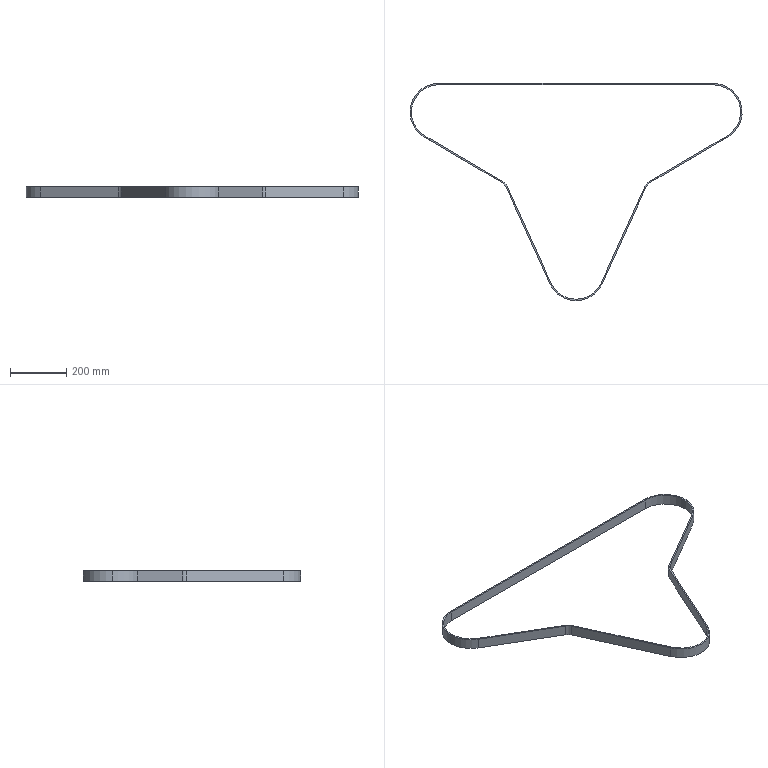Part | SolidWorks | features BeltProfileFeature 1, ExtruThin 1 | 1 solid | 24 faces | box 1186 x 775.76 x 38 mm | volume 604622 mm3 | cylinder 12 | plane 12 | commonest cylinder face diameters 195.76 x4 205.76 x4 65 x2 75 x2
STEP:
#1=CARTESIAN_POINT('',(-490.,667.88,19.));
#2=VERTEX_POINT('',#1);
#3=CARTESIAN_POINT('',(-587.88,570.,19.));
#4=VERTEX_POINT('',#3);
#5=CARTESIAN_POINT('',(-490.,570.,19.));
#6=DIRECTION('',(0.,0.,1.));
#7=DIRECTION('',(-1.,0.,0.));
#8=AXIS2_PLACEMENT_3D('',#5,#6,#7);
#9=CIRCLE('',#8,97.88);
#10=EDGE_CURVE('',#2,#4,#9,.T.);
#11=ORIENTED_EDGE('',*,*,#10,.T.);
#12=CARTESIAN_POINT('',(-587.88,570.,-19.));
#13=VERTEX_POINT('',#12);
#14=CARTESIAN_POINT('',(-587.88,570.,19.));
#15=DIRECTION('',(0.,0.,-1.));
#16=VECTOR('',#15,1000.);
#17=LINE('',#14,#16);
#18=EDGE_CURVE('',#4,#13,#17,.T.);
#19=ORIENTED_EDGE('',*,*,#18,.T.);
#20=CARTESIAN_POINT('',(-490.,667.88,-19.));
#21=VERTEX_POINT('',#20);
#22=CARTESIAN_POINT('',(-490.,570.,-19.));
#23=DIRECTION('',(0.,0.,1.));
#24=DIRECTION('',(-1.,0.,0.));
#25=AXIS2_PLACEMENT_3D('',#22,#23,#24);
#26=CIRCLE('',#25,97.88);
#27=EDGE_CURVE('',#21,#13,#26,.T.);
#28=ORIENTED_EDGE('',*,*,#27,.F.);
#29=CARTESIAN_POINT('',(-490.,667.88,19.));
#30=DIRECTION('',(0.,0.,-1.));
#31=VECTOR('',#30,1000.);
#32=LINE('',#29,#31);
#33=EDGE_CURVE('',#2,#21,#32,.T.);
#34=ORIENTED_EDGE('',*,*,#33,.F.);
#35=EDGE_LOOP('',(#11,#19,#28,#34));
#36=FACE_OUTER_BOUND('',#35,.T.);
#37=CARTESIAN_POINT('',(-490.,570.,19.));
#38=DIRECTION('',(0.,0.,-1.));
#39=DIRECTION('',(-1.,0.,0.));
#40=AXIS2_PLACEMENT_3D('',#37,#38,#39);
#41=CYLINDRICAL_SURFACE('',#40,97.88);
#42=ADVANCED_FACE('',(#36),#41,.F.);
#43=CARTESIAN_POINT('',(-592.88,570.,19.));
#44=VERTEX_POINT('',#43);
#45=CARTESIAN_POINT('',(-542.021,481.241,19.));
#46=VERTEX_POINT('',#45);
#47=CARTESIAN_POINT('',(-490.,570.,19.));
#48=DIRECTION('',(0.,0.,1.));
#49=DIRECTION('',(-1.,0.,0.));
#50=AXIS2_PLACEMENT_3D('',#47,#48,#49);
#51=CIRCLE('',#50,102.88);
#52=EDGE_CURVE('',#44,#46,#51,.T.);
#53=ORIENTED_EDGE('',*,*,#52,.F.);
#54=CARTESIAN_POINT('',(-592.88,570.,-19.));
#55=VERTEX_POINT('',#54);
#56=CARTESIAN_POINT('',(-592.88,570.,19.));
#57=DIRECTION('',(0.,0.,-1.));
#58=VECTOR('',#57,1000.);
#59=LINE('',#56,#58);
#60=EDGE_CURVE('',#44,#55,#59,.T.);
#61=ORIENTED_EDGE('',*,*,#60,.T.);
#62=CARTESIAN_POINT('',(-542.021,481.241,-19.));
#63=VERTEX_POINT('',#62);
#64=CARTESIAN_POINT('',(-490.,570.,-19.));
#65=DIRECTION('',(0.,0.,1.));
#66=DIRECTION('',(-1.,0.,0.));
#67=AXIS2_PLACEMENT_3D('',#64,#65,#66);
#68=CIRCLE('',#67,102.88);
#69=EDGE_CURVE('',#55,#63,#68,.T.);
#70=ORIENTED_EDGE('',*,*,#69,.T.);
#71=CARTESIAN_POINT('',(-542.021,481.241,19.));
#72=DIRECTION('',(0.,0.,-1.));
#73=VECTOR('',#72,1000.);
#74=LINE('',#71,#73);
#75=EDGE_CURVE('',#46,#63,#74,.T.);
#76=ORIENTED_EDGE('',*,*,#75,.F.);
#77=EDGE_LOOP('',(#53,#61,#70,#76));
#78=FACE_OUTER_BOUND('',#77,.T.);
#79=CARTESIAN_POINT('',(-490.,570.,19.));
#80=DIRECTION('',(0.,0.,-1.));
#81=DIRECTION('',(-1.,0.,0.));
#82=AXIS2_PLACEMENT_3D('',#79,#80,#81);
#83=CYLINDRICAL_SURFACE('',#82,102.88);
#84=ADVANCED_FACE('',(#78),#83,.T.);
#85=CARTESIAN_POINT('',(-93.712,-42.454,19.));
#86=VERTEX_POINT('',#85);
#87=CARTESIAN_POINT('',(93.712,-42.454,19.));
#88=VERTEX_POINT('',#87);
#89=CARTESIAN_POINT('',(0.,-0.00002578,19.));
#90=DIRECTION('',(0.,0.,1.));
#91=DIRECTION('',(-1.,0.,0.));
#92=AXIS2_PLACEMENT_3D('',#89,#90,#91);
#93=CIRCLE('',#92,102.88);
#94=EDGE_CURVE('',#86,#88,#93,.T.);
#95=ORIENTED_EDGE('',*,*,#94,.T.);
#96=CARTESIAN_POINT('',(250.396,303.411,19.));
#97=VERTEX_POINT('',#96);
#98=CARTESIAN_POINT('',(93.712,-42.454,19.));
#99=DIRECTION('',(0.4127,0.9109,0.));
#100=VECTOR('',#99,1000.);
#101=LINE('',#98,#100);
#102=EDGE_CURVE('',#88,#97,#101,.T.);
#103=ORIENTED_EDGE('',*,*,#102,.T.);
#104=CARTESIAN_POINT('',(263.566,318.039,19.));
#105=VERTEX_POINT('',#104);
#106=CARTESIAN_POINT('',(280.,290.,19.));
#107=DIRECTION('',(0.,0.,-1.));
#108=DIRECTION('',(-1.,0.,0.));
#109=AXIS2_PLACEMENT_3D('',#106,#107,#108);
#110=CIRCLE('',#109,32.5);
#111=EDGE_CURVE('',#97,#105,#110,.T.);
#112=ORIENTED_EDGE('',*,*,#111,.T.);
#113=CARTESIAN_POINT('',(542.021,481.241,19.));
#114=VERTEX_POINT('',#113);
#115=CARTESIAN_POINT('',(-71.353,121.743,19.));
#116=DIRECTION('',(0.8627,0.5057,0.));
#117=VECTOR('',#116,1000.);
#118=LINE('',#115,#117);
#119=EDGE_CURVE('',#105,#114,#118,.T.);
#120=ORIENTED_EDGE('',*,*,#119,.T.);
#121=CARTESIAN_POINT('',(490.,672.88,19.));
#122=VERTEX_POINT('',#121);
#123=CARTESIAN_POINT('',(490.,570.,19.));
#124=DIRECTION('',(0.,0.,1.));
#125=DIRECTION('',(-1.,0.,0.));
#126=AXIS2_PLACEMENT_3D('',#123,#124,#125);
#127=CIRCLE('',#126,102.88);
#128=EDGE_CURVE('',#114,#122,#127,.T.);
#129=ORIENTED_EDGE('',*,*,#128,.T.);
#130=CARTESIAN_POINT('',(-490.,672.88,19.));
#131=VERTEX_POINT('',#130);
#132=CARTESIAN_POINT('',(0.,672.88,19.));
#133=DIRECTION('',(-1.,0.,0.));
#134=VECTOR('',#133,1000.);
#135=LINE('',#132,#134);
#136=EDGE_CURVE('',#122,#131,#135,.T.);
#137=ORIENTED_EDGE('',*,*,#136,.T.);
#138=CARTESIAN_POINT('',(-490.,570.,19.));
#139=DIRECTION('',(0.,0.,1.));
#140=DIRECTION('',(-1.,0.,0.));
#141=AXIS2_PLACEMENT_3D('',#138,#139,#140);
#142=CIRCLE('',#141,102.88);
#143=EDGE_CURVE('',#131,#44,#142,.T.);
#144=ORIENTED_EDGE('',*,*,#143,.T.);
#145=ORIENTED_EDGE('',*,*,#52,.T.);
#146=CARTESIAN_POINT('',(-263.566,318.039,19.));
#147=VERTEX_POINT('',#146);
#148=CARTESIAN_POINT('',(71.353,121.743,19.));
#149=DIRECTION('',(0.8627,-0.5057,0.));
#150=VECTOR('',#149,1000.);
#151=LINE('',#148,#150);
#152=EDGE_CURVE('',#46,#147,#151,.T.);
#153=ORIENTED_EDGE('',*,*,#152,.T.);
#154=CARTESIAN_POINT('',(-250.396,303.411,19.));
#155=VERTEX_POINT('',#154);
#156=CARTESIAN_POINT('',(-280.,290.,19.));
#157=DIRECTION('',(0.,0.,-1.));
#158=DIRECTION('',(-1.,0.,0.));
#159=AXIS2_PLACEMENT_3D('',#156,#157,#158);
#160=CIRCLE('',#159,32.5);
#161=EDGE_CURVE('',#147,#155,#160,.T.);
#162=ORIENTED_EDGE('',*,*,#161,.T.);
#163=CARTESIAN_POINT('',(-93.712,-42.454,19.));
#164=DIRECTION('',(0.4127,-0.9109,0.));
#165=VECTOR('',#164,1000.);
#166=LINE('',#163,#165);
#167=EDGE_CURVE('',#155,#86,#166,.T.);
#168=ORIENTED_EDGE('',*,*,#167,.T.);
#169=EDGE_LOOP('',(#95,#103,#112,#120,#129,#137,#144,#145,#153,#162,#168));
#170=FACE_OUTER_BOUND('',#169,.T.);
#171=CARTESIAN_POINT('',(-89.158,-40.39,19.));
#172=VERTEX_POINT('',#171);
#173=CARTESIAN_POINT('',(89.158,-40.39,19.));
#174=VERTEX_POINT('',#173);
#175=CARTESIAN_POINT('',(0.,-0.00002578,19.));
#176=DIRECTION('',(0.,0.,1.));
#177=DIRECTION('',(-1.,0.,0.));
#178=AXIS2_PLACEMENT_3D('',#175,#176,#177);
#179=CIRCLE('',#178,97.88);
#180=EDGE_CURVE('',#172,#174,#179,.T.);
#181=ORIENTED_EDGE('',*,*,#180,.F.);
#182=CARTESIAN_POINT('',(-245.842,305.474,19.));
#183=VERTEX_POINT('',#182);
#184=CARTESIAN_POINT('',(-89.158,-40.39,19.));
#185=DIRECTION('',(0.4127,-0.9109,0.));
#186=VECTOR('',#185,1000.);
#187=LINE('',#184,#186);
#188=EDGE_CURVE('',#183,#172,#187,.T.);
#189=ORIENTED_EDGE('',*,*,#188,.F.);
#190=CARTESIAN_POINT('',(-261.038,322.353,19.));
#191=VERTEX_POINT('',#190);
#192=CARTESIAN_POINT('',(-280.,290.,19.));
#193=DIRECTION('',(0.,0.,-1.));
#194=DIRECTION('',(-1.,0.,0.));
#195=AXIS2_PLACEMENT_3D('',#192,#193,#194);
#196=CIRCLE('',#195,37.5);
#197=EDGE_CURVE('',#191,#183,#196,.T.);
#198=ORIENTED_EDGE('',*,*,#197,.F.);
#199=CARTESIAN_POINT('',(-539.493,485.555,19.));
#200=VERTEX_POINT('',#199);
#201=CARTESIAN_POINT('',(73.882,126.056,19.));
#202=DIRECTION('',(0.8627,-0.5057,0.));
#203=VECTOR('',#202,1000.);
#204=LINE('',#201,#203);
#205=EDGE_CURVE('',#200,#191,#204,.T.);
#206=ORIENTED_EDGE('',*,*,#205,.F.);
#207=CARTESIAN_POINT('',(-490.,570.,19.));
#208=DIRECTION('',(0.,0.,1.));
#209=DIRECTION('',(-1.,0.,0.));
#210=AXIS2_PLACEMENT_3D('',#207,#208,#209);
#211=CIRCLE('',#210,97.88);
#212=EDGE_CURVE('',#4,#200,#211,.T.);
#213=ORIENTED_EDGE('',*,*,#212,.F.);
#214=ORIENTED_EDGE('',*,*,#10,.F.);
#215=CARTESIAN_POINT('',(490.,667.88,19.));
#216=VERTEX_POINT('',#215);
#217=CARTESIAN_POINT('',(0.,667.88,19.));
#218=DIRECTION('',(-1.,0.,0.));
#219=VECTOR('',#218,1000.);
#220=LINE('',#217,#219);
#221=EDGE_CURVE('',#216,#2,#220,.T.);
#222=ORIENTED_EDGE('',*,*,#221,.F.);
#223=CARTESIAN_POINT('',(539.493,485.555,19.));
#224=VERTEX_POINT('',#223);
#225=CARTESIAN_POINT('',(490.,570.,19.));
#226=DIRECTION('',(0.,0.,1.));
#227=DIRECTION('',(-1.,0.,0.));
#228=AXIS2_PLACEMENT_3D('',#225,#226,#227);
#229=CIRCLE('',#228,97.88);
#230=EDGE_CURVE('',#224,#216,#229,.T.);
#231=ORIENTED_EDGE('',*,*,#230,.F.);
#232=CARTESIAN_POINT('',(261.038,322.353,19.));
#233=VERTEX_POINT('',#232);
#234=CARTESIAN_POINT('',(-73.882,126.056,19.));
#235=DIRECTION('',(0.8627,0.5057,0.));
#236=VECTOR('',#235,1000.);
#237=LINE('',#234,#236);
#238=EDGE_CURVE('',#233,#224,#237,.T.);
#239=ORIENTED_EDGE('',*,*,#238,.F.);
#240=CARTESIAN_POINT('',(245.842,305.474,19.));
#241=VERTEX_POINT('',#240);
#242=CARTESIAN_POINT('',(280.,290.,19.));
#243=DIRECTION('',(0.,0.,-1.));
#244=DIRECTION('',(-1.,0.,0.));
#245=AXIS2_PLACEMENT_3D('',#242,#243,#244);
#246=CIRCLE('',#245,37.5);
#247=EDGE_CURVE('',#241,#233,#246,.T.);
#248=ORIENTED_EDGE('',*,*,#247,.F.);
#249=CARTESIAN_POINT('',(89.158,-40.39,19.));
#250=DIRECTION('',(0.4127,0.9109,0.));
#251=VECTOR('',#250,1000.);
#252=LINE('',#249,#251);
#253=EDGE_CURVE('',#174,#241,#252,.T.);
#254=ORIENTED_EDGE('',*,*,#253,.F.);
#255=EDGE_LOOP('',(#181,#189,#198,#206,#213,#214,#222,#231,#239,#248,#254));
#256=FACE_BOUND('',#255,.T.);
#257=CARTESIAN_POINT('',(0.,-0.00002578,19.));
#258=DIRECTION('',(0.,0.,-1.));
#259=DIRECTION('',(-1.,0.,0.));
#260=AXIS2_PLACEMENT_3D('',#257,#258,#259);
#261=PLANE('',#260);
#262=ADVANCED_FACE('',(#170,#256),#261,.F.);
#263=CARTESIAN_POINT('',(-93.712,-42.454,-19.));
#264=VERTEX_POINT('',#263);
#265=CARTESIAN_POINT('',(93.712,-42.454,-19.));
#266=VERTEX_POINT('',#265);
#267=CARTESIAN_POINT('',(0.,-0.00002578,-19.));
#268=DIRECTION('',(0.,0.,1.));
#269=DIRECTION('',(-1.,0.,0.));
#270=AXIS2_PLACEMENT_3D('',#267,#268,#269);
#271=CIRCLE('',#270,102.88);
#272=EDGE_CURVE('',#264,#266,#271,.T.);
#273=ORIENTED_EDGE('',*,*,#272,.F.);
#274=CARTESIAN_POINT('',(-250.396,303.411,-19.));
#275=VERTEX_POINT('',#274);
#276=CARTESIAN_POINT('',(-93.712,-42.454,-19.));
#277=DIRECTION('',(0.4127,-0.9109,0.));
#278=VECTOR('',#277,1000.);
#279=LINE('',#276,#278);
#280=EDGE_CURVE('',#275,#264,#279,.T.);
#281=ORIENTED_EDGE('',*,*,#280,.F.);
#282=CARTESIAN_POINT('',(-263.566,318.039,-19.));
#283=VERTEX_POINT('',#282);
#284=CARTESIAN_POINT('',(-280.,290.,-19.));
#285=DIRECTION('',(0.,0.,-1.));
#286=DIRECTION('',(-1.,0.,0.));
#287=AXIS2_PLACEMENT_3D('',#284,#285,#286);
#288=CIRCLE('',#287,32.5);
#289=EDGE_CURVE('',#283,#275,#288,.T.);
#290=ORIENTED_EDGE('',*,*,#289,.F.);
#291=CARTESIAN_POINT('',(71.353,121.743,-19.));
#292=DIRECTION('',(0.8627,-0.5057,0.));
#293=VECTOR('',#292,1000.);
#294=LINE('',#291,#293);
#295=EDGE_CURVE('',#63,#283,#294,.T.);
#296=ORIENTED_EDGE('',*,*,#295,.F.);
#297=ORIENTED_EDGE('',*,*,#69,.F.);
#298=CARTESIAN_POINT('',(-490.,672.88,-19.));
#299=VERTEX_POINT('',#298);
#300=CARTESIAN_POINT('',(-490.,570.,-19.));
#301=DIRECTION('',(0.,0.,1.));
#302=DIRECTION('',(-1.,0.,0.));
#303=AXIS2_PLACEMENT_3D('',#300,#301,#302);
#304=CIRCLE('',#303,102.88);
#305=EDGE_CURVE('',#299,#55,#304,.T.);
#306=ORIENTED_EDGE('',*,*,#305,.F.);
#307=CARTESIAN_POINT('',(490.,672.88,-19.));
#308=VERTEX_POINT('',#307);
#309=CARTESIAN_POINT('',(0.,672.88,-19.));
#310=DIRECTION('',(-1.,0.,0.));
#311=VECTOR('',#310,1000.);
#312=LINE('',#309,#311);
#313=EDGE_CURVE('',#308,#299,#312,.T.);
#314=ORIENTED_EDGE('',*,*,#313,.F.);
#315=CARTESIAN_POINT('',(542.021,481.241,-19.));
#316=VERTEX_POINT('',#315);
#317=CARTESIAN_POINT('',(490.,570.,-19.));
#318=DIRECTION('',(0.,0.,1.));
#319=DIRECTION('',(-1.,0.,0.));
#320=AXIS2_PLACEMENT_3D('',#317,#318,#319);
#321=CIRCLE('',#320,102.88);
#322=EDGE_CURVE('',#316,#308,#321,.T.);
#323=ORIENTED_EDGE('',*,*,#322,.F.);
#324=CARTESIAN_POINT('',(263.566,318.039,-19.));
#325=VERTEX_POINT('',#324);
#326=CARTESIAN_POINT('',(-71.353,121.743,-19.));
#327=DIRECTION('',(0.8627,0.5057,0.));
#328=VECTOR('',#327,1000.);
#329=LINE('',#326,#328);
#330=EDGE_CURVE('',#325,#316,#329,.T.);
#331=ORIENTED_EDGE('',*,*,#330,.F.);
#332=CARTESIAN_POINT('',(250.396,303.411,-19.));
#333=VERTEX_POINT('',#332);
#334=CARTESIAN_POINT('',(280.,290.,-19.));
#335=DIRECTION('',(0.,0.,-1.));
#336=DIRECTION('',(-1.,0.,0.));
#337=AXIS2_PLACEMENT_3D('',#334,#335,#336);
#338=CIRCLE('',#337,32.5);
#339=EDGE_CURVE('',#333,#325,#338,.T.);
#340=ORIENTED_EDGE('',*,*,#339,.F.);
#341=CARTESIAN_POINT('',(93.712,-42.454,-19.));
#342=DIRECTION('',(0.4127,0.9109,0.));
#343=VECTOR('',#342,1000.);
#344=LINE('',#341,#343);
#345=EDGE_CURVE('',#266,#333,#344,.T.);
#346=ORIENTED_EDGE('',*,*,#345,.F.);
#347=EDGE_LOOP('',(#273,#281,#290,#296,#297,#306,#314,#323,#331,#340,#346));
#348=FACE_OUTER_BOUND('',#347,.T.);
#349=CARTESIAN_POINT('',(-245.842,305.474,-19.));
#350=VERTEX_POINT('',#349);
#351=CARTESIAN_POINT('',(-89.158,-40.39,-19.));
#352=VERTEX_POINT('',#351);
#353=CARTESIAN_POINT('',(-89.158,-40.39,-19.));
#354=DIRECTION('',(0.4127,-0.9109,0.));
#355=VECTOR('',#354,1000.);
#356=LINE('',#353,#355);
#357=EDGE_CURVE('',#350,#352,#356,.T.);
#358=ORIENTED_EDGE('',*,*,#357,.T.);
#359=CARTESIAN_POINT('',(89.158,-40.39,-19.));
#360=VERTEX_POINT('',#359);
#361=CARTESIAN_POINT('',(0.,-0.00002578,-19.));
#362=DIRECTION('',(0.,0.,1.));
#363=DIRECTION('',(-1.,0.,0.));
#364=AXIS2_PLACEMENT_3D('',#361,#362,#363);
#365=CIRCLE('',#364,97.88);
#366=EDGE_CURVE('',#352,#360,#365,.T.);
#367=ORIENTED_EDGE('',*,*,#366,.T.);
#368=CARTESIAN_POINT('',(245.842,305.474,-19.));
#369=VERTEX_POINT('',#368);
#370=CARTESIAN_POINT('',(89.158,-40.39,-19.));
#371=DIRECTION('',(0.4127,0.9109,0.));
#372=VECTOR('',#371,1000.);
#373=LINE('',#370,#372);
#374=EDGE_CURVE('',#360,#369,#373,.T.);
#375=ORIENTED_EDGE('',*,*,#374,.T.);
#376=CARTESIAN_POINT('',(261.038,322.353,-19.));
#377=VERTEX_POINT('',#376);
#378=CARTESIAN_POINT('',(280.,290.,-19.));
#379=DIRECTION('',(0.,0.,-1.));
#380=DIRECTION('',(-1.,0.,0.));
#381=AXIS2_PLACEMENT_3D('',#378,#379,#380);
#382=CIRCLE('',#381,37.5);
#383=EDGE_CURVE('',#369,#377,#382,.T.);
#384=ORIENTED_EDGE('',*,*,#383,.T.);
#385=CARTESIAN_POINT('',(539.493,485.555,-19.));
#386=VERTEX_POINT('',#385);
#387=CARTESIAN_POINT('',(-73.882,126.056,-19.));
#388=DIRECTION('',(0.8627,0.5057,0.));
#389=VECTOR('',#388,1000.);
#390=LINE('',#387,#389);
#391=EDGE_CURVE('',#377,#386,#390,.T.);
#392=ORIENTED_EDGE('',*,*,#391,.T.);
#393=CARTESIAN_POINT('',(490.,667.88,-19.));
#394=VERTEX_POINT('',#393);
#395=CARTESIAN_POINT('',(490.,570.,-19.));
#396=DIRECTION('',(0.,0.,1.));
#397=DIRECTION('',(-1.,0.,0.));
#398=AXIS2_PLACEMENT_3D('',#395,#396,#397);
#399=CIRCLE('',#398,97.88);
#400=EDGE_CURVE('',#386,#394,#399,.T.);
#401=ORIENTED_EDGE('',*,*,#400,.T.);
#402=CARTESIAN_POINT('',(0.,667.88,-19.));
#403=DIRECTION('',(-1.,0.,0.));
#404=VECTOR('',#403,1000.);
#405=LINE('',#402,#404);
#406=EDGE_CURVE('',#394,#21,#405,.T.);
#407=ORIENTED_EDGE('',*,*,#406,.T.);
#408=ORIENTED_EDGE('',*,*,#27,.T.);
#409=CARTESIAN_POINT('',(-539.493,485.555,-19.));
#410=VERTEX_POINT('',#409);
#411=CARTESIAN_POINT('',(-490.,570.,-19.));
#412=DIRECTION('',(0.,0.,1.));
#413=DIRECTION('',(-1.,0.,0.));
#414=AXIS2_PLACEMENT_3D('',#411,#412,#413);
#415=CIRCLE('',#414,97.88);
#416=EDGE_CURVE('',#13,#410,#415,.T.);
#417=ORIENTED_EDGE('',*,*,#416,.T.);
#418=CARTESIAN_POINT('',(-261.038,322.353,-19.));
#419=VERTEX_POINT('',#418);
#420=CARTESIAN_POINT('',(73.882,126.056,-19.));
#421=DIRECTION('',(0.8627,-0.5057,0.));
#422=VECTOR('',#421,1000.);
#423=LINE('',#420,#422);
#424=EDGE_CURVE('',#410,#419,#423,.T.);
#425=ORIENTED_EDGE('',*,*,#424,.T.);
#426=CARTESIAN_POINT('',(-280.,290.,-19.));
#427=DIRECTION('',(0.,0.,-1.));
#428=DIRECTION('',(-1.,0.,0.));
#429=AXIS2_PLACEMENT_3D('',#426,#427,#428);
#430=CIRCLE('',#429,37.5);
#431=EDGE_CURVE('',#419,#350,#430,.T.);
#432=ORIENTED_EDGE('',*,*,#431,.T.);
#433=EDGE_LOOP('',(#358,#367,#375,#384,#392,#401,#407,#408,#417,#425,#432));
#434=FACE_BOUND('',#433,.T.);
#435=CARTESIAN_POINT('',(0.,-0.00002578,-19.));
#436=DIRECTION('',(0.,0.,-1.));
#437=DIRECTION('',(-1.,0.,0.));
#438=AXIS2_PLACEMENT_3D('',#435,#436,#437);
#439=PLANE('',#438);
#440=ADVANCED_FACE('',(#348,#434),#439,.T.);
#441=ORIENTED_EDGE('',*,*,#272,.T.);
#442=CARTESIAN_POINT('',(93.712,-42.454,19.));
#443=DIRECTION('',(0.,0.,-1.));
#444=VECTOR('',#443,1000.);
#445=LINE('',#442,#444);
#446=EDGE_CURVE('',#88,#266,#445,.T.);
#447=ORIENTED_EDGE('',*,*,#446,.F.);
#448=ORIENTED_EDGE('',*,*,#94,.F.);
#449=CARTESIAN_POINT('',(-93.712,-42.454,19.));
#450=DIRECTION('',(0.,0.,-1.));
#451=VECTOR('',#450,1000.);
#452=LINE('',#449,#451);
#453=EDGE_CURVE('',#86,#264,#452,.T.);
#454=ORIENTED_EDGE('',*,*,#453,.T.);
#455=EDGE_LOOP('',(#441,#447,#448,#454));
#456=FACE_OUTER_BOUND('',#455,.T.);
#457=CARTESIAN_POINT('',(0.,-0.00002578,19.));
#458=DIRECTION('',(0.,0.,-1.));
#459=DIRECTION('',(-1.,0.,0.));
#460=AXIS2_PLACEMENT_3D('',#457,#458,#459);
#461=CYLINDRICAL_SURFACE('',#460,102.88);
#462=ADVANCED_FACE('',(#456),#461,.T.);
#463=ORIENTED_EDGE('',*,*,#345,.T.);
#464=CARTESIAN_POINT('',(250.396,303.411,19.));
#465=DIRECTION('',(0.,0.,-1.));
#466=VECTOR('',#465,1000.);
#467=LINE('',#464,#466);
#468=EDGE_CURVE('',#97,#333,#467,.T.);
#469=ORIENTED_EDGE('',*,*,#468,.F.);
#470=ORIENTED_EDGE('',*,*,#102,.F.);
#471=ORIENTED_EDGE('',*,*,#446,.T.);
#472=EDGE_LOOP('',(#463,#469,#470,#471));
#473=FACE_OUTER_BOUND('',#472,.T.);
#474=CARTESIAN_POINT('',(93.712,-42.454,19.));
#475=DIRECTION('',(-0.9109,0.4127,0.));
#476=DIRECTION('',(-0.4127,-0.9109,0.));
#477=AXIS2_PLACEMENT_3D('',#474,#475,#476);
#478=PLANE('',#477);
#479=ADVANCED_FACE('',(#473),#478,.F.);
#480=ORIENTED_EDGE('',*,*,#339,.T.);
#481=CARTESIAN_POINT('',(263.566,318.039,19.));
#482=DIRECTION('',(0.,0.,-1.));
#483=VECTOR('',#482,1000.);
#484=LINE('',#481,#483);
#485=EDGE_CURVE('',#105,#325,#484,.T.);
#486=ORIENTED_EDGE('',*,*,#485,.F.);
#487=ORIENTED_EDGE('',*,*,#111,.F.);
#488=ORIENTED_EDGE('',*,*,#468,.T.);
#489=EDGE_LOOP('',(#480,#486,#487,#488));
#490=FACE_OUTER_BOUND('',#489,.T.);
#491=CARTESIAN_POINT('',(280.,290.,19.));
#492=DIRECTION('',(0.,0.,-1.));
#493=DIRECTION('',(-1.,0.,0.));
#494=AXIS2_PLACEMENT_3D('',#491,#492,#493);
#495=CYLINDRICAL_SURFACE('',#494,32.5);
#496=ADVANCED_FACE('',(#490),#495,.F.);
#497=ORIENTED_EDGE('',*,*,#330,.T.);
#498=CARTESIAN_POINT('',(542.021,481.241,19.));
#499=DIRECTION('',(0.,0.,-1.));
#500=VECTOR('',#499,1000.);
#501=LINE('',#498,#500);
#502=EDGE_CURVE('',#114,#316,#501,.T.);
#503=ORIENTED_EDGE('',*,*,#502,.F.);
#504=ORIENTED_EDGE('',*,*,#119,.F.);
#505=ORIENTED_EDGE('',*,*,#485,.T.);
#506=EDGE_LOOP('',(#497,#503,#504,#505));
#507=FACE_OUTER_BOUND('',#506,.T.);
#508=CARTESIAN_POINT('',(-71.353,121.743,19.));
#509=DIRECTION('',(-0.5057,0.8627,0.));
#510=DIRECTION('',(-0.8627,-0.5057,0.));
#511=AXIS2_PLACEMENT_3D('',#508,#509,#510);
#512=PLANE('',#511);
#513=ADVANCED_FACE('',(#507),#512,.F.);
#514=ORIENTED_EDGE('',*,*,#322,.T.);
#515=CARTESIAN_POINT('',(490.,672.88,19.));
#516=DIRECTION('',(0.,0.,-1.));
#517=VECTOR('',#516,1000.);
#518=LINE('',#515,#517);
#519=EDGE_CURVE('',#122,#308,#518,.T.);
#520=ORIENTED_EDGE('',*,*,#519,.F.);
#521=ORIENTED_EDGE('',*,*,#128,.F.);
#522=ORIENTED_EDGE('',*,*,#502,.T.);
#523=EDGE_LOOP('',(#514,#520,#521,#522));
#524=FACE_OUTER_BOUND('',#523,.T.);
#525=CARTESIAN_POINT('',(490.,570.,19.));
#526=DIRECTION('',(0.,0.,-1.));
#527=DIRECTION('',(-1.,0.,0.));
#528=AXIS2_PLACEMENT_3D('',#525,#526,#527);
#529=CYLINDRICAL_SURFACE('',#528,102.88);
#530=ADVANCED_FACE('',(#524),#529,.T.);
#531=ORIENTED_EDGE('',*,*,#313,.T.);
#532=CARTESIAN_POINT('',(-490.,672.88,19.));
#533=DIRECTION('',(0.,0.,-1.));
#534=VECTOR('',#533,1000.);
#535=LINE('',#532,#534);
#536=EDGE_CURVE('',#131,#299,#535,.T.);
#537=ORIENTED_EDGE('',*,*,#536,.F.);
#538=ORIENTED_EDGE('',*,*,#136,.F.);
#539=ORIENTED_EDGE('',*,*,#519,.T.);
#540=EDGE_LOOP('',(#531,#537,#538,#539));
#541=FACE_OUTER_BOUND('',#540,.T.);
#542=CARTESIAN_POINT('',(0.,672.88,19.));
#543=DIRECTION('',(0.,-1.,0.));
#544=DIRECTION('',(1.,0.,0.));
#545=AXIS2_PLACEMENT_3D('',#542,#543,#544);
#546=PLANE('',#545);
#547=ADVANCED_FACE('',(#541),#546,.F.);
#548=ORIENTED_EDGE('',*,*,#60,.F.);
#549=ORIENTED_EDGE('',*,*,#143,.F.);
#550=ORIENTED_EDGE('',*,*,#536,.T.);
#551=ORIENTED_EDGE('',*,*,#305,.T.);
#552=EDGE_LOOP('',(#548,#549,#550,#551));
#553=FACE_OUTER_BOUND('',#552,.T.);
#554=CARTESIAN_POINT('',(-490.,570.,19.));
#555=DIRECTION('',(0.,0.,-1.));
#556=DIRECTION('',(-1.,0.,0.));
#557=AXIS2_PLACEMENT_3D('',#554,#555,#556);
#558=CYLINDRICAL_SURFACE('',#557,102.88);
#559=ADVANCED_FACE('',(#553),#558,.T.);
#560=ORIENTED_EDGE('',*,*,#295,.T.);
#561=CARTESIAN_POINT('',(-263.566,318.039,19.));
#562=DIRECTION('',(0.,0.,-1.));
#563=VECTOR('',#562,1000.);
#564=LINE('',#561,#563);
#565=EDGE_CURVE('',#147,#283,#564,.T.);
#566=ORIENTED_EDGE('',*,*,#565,.F.);
#567=ORIENTED_EDGE('',*,*,#152,.F.);
#568=ORIENTED_EDGE('',*,*,#75,.T.);
#569=EDGE_LOOP('',(#560,#566,#567,#568));
#570=FACE_OUTER_BOUND('',#569,.T.);
#571=CARTESIAN_POINT('',(71.353,121.743,19.));
#572=DIRECTION('',(0.5057,0.8627,0.));
#573=DIRECTION('',(-0.8627,0.5057,0.));
#574=AXIS2_PLACEMENT_3D('',#571,#572,#573);
#575=PLANE('',#574);
#576=ADVANCED_FACE('',(#570),#575,.F.);
#577=ORIENTED_EDGE('',*,*,#289,.T.);
#578=CARTESIAN_POINT('',(-250.396,303.411,19.));
#579=DIRECTION('',(0.,0.,-1.));
#580=VECTOR('',#579,1000.);
#581=LINE('',#578,#580);
#582=EDGE_CURVE('',#155,#275,#581,.T.);
#583=ORIENTED_EDGE('',*,*,#582,.F.);
#584=ORIENTED_EDGE('',*,*,#161,.F.);
#585=ORIENTED_EDGE('',*,*,#565,.T.);
#586=EDGE_LOOP('',(#577,#583,#584,#585));
#587=FACE_OUTER_BOUND('',#586,.T.);
#588=CARTESIAN_POINT('',(-280.,290.,19.));
#589=DIRECTION('',(0.,0.,-1.));
#590=DIRECTION('',(-1.,0.,0.));
#591=AXIS2_PLACEMENT_3D('',#588,#589,#590);
#592=CYLINDRICAL_SURFACE('',#591,32.5);
#593=ADVANCED_FACE('',(#587),#592,.F.);
#594=ORIENTED_EDGE('',*,*,#280,.T.);
#595=ORIENTED_EDGE('',*,*,#453,.F.);
#596=ORIENTED_EDGE('',*,*,#167,.F.);
#597=ORIENTED_EDGE('',*,*,#582,.T.);
#598=EDGE_LOOP('',(#594,#595,#596,#597));
#599=FACE_OUTER_BOUND('',#598,.T.);
#600=CARTESIAN_POINT('',(-93.712,-42.454,19.));
#601=DIRECTION('',(0.9109,0.4127,0.));
#602=DIRECTION('',(-0.4127,0.9109,0.));
#603=AXIS2_PLACEMENT_3D('',#600,#601,#602);
#604=PLANE('',#603);
#605=ADVANCED_FACE('',(#599),#604,.F.);
#606=ORIENTED_EDGE('',*,*,#366,.F.);
#607=CARTESIAN_POINT('',(-89.158,-40.39,19.));
#608=DIRECTION('',(0.,0.,-1.));
#609=VECTOR('',#608,1000.);
#610=LINE('',#607,#609);
#611=EDGE_CURVE('',#172,#352,#610,.T.);
#612=ORIENTED_EDGE('',*,*,#611,.F.);
#613=ORIENTED_EDGE('',*,*,#180,.T.);
#614=CARTESIAN_POINT('',(89.158,-40.39,19.));
#615=DIRECTION('',(0.,0.,-1.));
#616=VECTOR('',#615,1000.);
#617=LINE('',#614,#616);
#618=EDGE_CURVE('',#174,#360,#617,.T.);
#619=ORIENTED_EDGE('',*,*,#618,.T.);
#620=EDGE_LOOP('',(#606,#612,#613,#619));
#621=FACE_OUTER_BOUND('',#620,.T.);
#622=CARTESIAN_POINT('',(0.,-0.00002578,19.));
#623=DIRECTION('',(0.,0.,-1.));
#624=DIRECTION('',(-1.,0.,0.));
#625=AXIS2_PLACEMENT_3D('',#622,#623,#624);
#626=CYLINDRICAL_SURFACE('',#625,97.88);
#627=ADVANCED_FACE('',(#621),#626,.F.);
#628=ORIENTED_EDGE('',*,*,#374,.F.);
#629=ORIENTED_EDGE('',*,*,#618,.F.);
#630=ORIENTED_EDGE('',*,*,#253,.T.);
#631=CARTESIAN_POINT('',(245.842,305.474,19.));
#632=DIRECTION('',(0.,0.,-1.));
#633=VECTOR('',#632,1000.);
#634=LINE('',#631,#633);
#635=EDGE_CURVE('',#241,#369,#634,.T.);
#636=ORIENTED_EDGE('',*,*,#635,.T.);
#637=EDGE_LOOP('',(#628,#629,#630,#636));
#638=FACE_OUTER_BOUND('',#637,.T.);
#639=CARTESIAN_POINT('',(89.158,-40.39,19.));
#640=DIRECTION('',(-0.9109,0.4127,0.));
#641=DIRECTION('',(-0.4127,-0.9109,0.));
#642=AXIS2_PLACEMENT_3D('',#639,#640,#641);
#643=PLANE('',#642);
#644=ADVANCED_FACE('',(#638),#643,.T.);
#645=ORIENTED_EDGE('',*,*,#383,.F.);
#646=ORIENTED_EDGE('',*,*,#635,.F.);
#647=ORIENTED_EDGE('',*,*,#247,.T.);
#648=CARTESIAN_POINT('',(261.038,322.353,19.));
#649=DIRECTION('',(0.,0.,-1.));
#650=VECTOR('',#649,1000.);
#651=LINE('',#648,#650);
#652=EDGE_CURVE('',#233,#377,#651,.T.);
#653=ORIENTED_EDGE('',*,*,#652,.T.);
#654=EDGE_LOOP('',(#645,#646,#647,#653));
#655=FACE_OUTER_BOUND('',#654,.T.);
#656=CARTESIAN_POINT('',(280.,290.,19.));
#657=DIRECTION('',(0.,0.,-1.));
#658=DIRECTION('',(-1.,0.,0.));
#659=AXIS2_PLACEMENT_3D('',#656,#657,#658);
#660=CYLINDRICAL_SURFACE('',#659,37.5);
#661=ADVANCED_FACE('',(#655),#660,.T.);
#662=ORIENTED_EDGE('',*,*,#391,.F.);
#663=ORIENTED_EDGE('',*,*,#652,.F.);
#664=ORIENTED_EDGE('',*,*,#238,.T.);
#665=CARTESIAN_POINT('',(539.493,485.555,19.));
#666=DIRECTION('',(0.,0.,-1.));
#667=VECTOR('',#666,1000.);
#668=LINE('',#665,#667);
#669=EDGE_CURVE('',#224,#386,#668,.T.);
#670=ORIENTED_EDGE('',*,*,#669,.T.);
#671=EDGE_LOOP('',(#662,#663,#664,#670));
#672=FACE_OUTER_BOUND('',#671,.T.);
#673=CARTESIAN_POINT('',(-73.882,126.056,19.));
#674=DIRECTION('',(-0.5057,0.8627,0.));
#675=DIRECTION('',(-0.8627,-0.5057,0.));
#676=AXIS2_PLACEMENT_3D('',#673,#674,#675);
#677=PLANE('',#676);
#678=ADVANCED_FACE('',(#672),#677,.T.);
#679=ORIENTED_EDGE('',*,*,#400,.F.);
#680=ORIENTED_EDGE('',*,*,#669,.F.);
#681=ORIENTED_EDGE('',*,*,#230,.T.);
#682=CARTESIAN_POINT('',(490.,667.88,19.));
#683=DIRECTION('',(0.,0.,-1.));
#684=VECTOR('',#683,1000.);
#685=LINE('',#682,#684);
#686=EDGE_CURVE('',#216,#394,#685,.T.);
#687=ORIENTED_EDGE('',*,*,#686,.T.);
#688=EDGE_LOOP('',(#679,#680,#681,#687));
#689=FACE_OUTER_BOUND('',#688,.T.);
#690=CARTESIAN_POINT('',(490.,570.,19.));
#691=DIRECTION('',(0.,0.,-1.));
#692=DIRECTION('',(-1.,0.,0.));
#693=AXIS2_PLACEMENT_3D('',#690,#691,#692);
#694=CYLINDRICAL_SURFACE('',#693,97.88);
#695=ADVANCED_FACE('',(#689),#694,.F.);
#696=ORIENTED_EDGE('',*,*,#406,.F.);
#697=ORIENTED_EDGE('',*,*,#686,.F.);
#698=ORIENTED_EDGE('',*,*,#221,.T.);
#699=ORIENTED_EDGE('',*,*,#33,.T.);
#700=EDGE_LOOP('',(#696,#697,#698,#699));
#701=FACE_OUTER_BOUND('',#700,.T.);
#702=CARTESIAN_POINT('',(0.,667.88,19.));
#703=DIRECTION('',(0.,-1.,0.));
#704=DIRECTION('',(1.,0.,0.));
#705=AXIS2_PLACEMENT_3D('',#702,#703,#704);
#706=PLANE('',#705);
#707=ADVANCED_FACE('',(#701),#706,.T.);
#708=ORIENTED_EDGE('',*,*,#18,.F.);
#709=ORIENTED_EDGE('',*,*,#212,.T.);
#710=CARTESIAN_POINT('',(-539.493,485.555,19.));
#711=DIRECTION('',(0.,0.,-1.));
#712=VECTOR('',#711,1000.);
#713=LINE('',#710,#712);
#714=EDGE_CURVE('',#200,#410,#713,.T.);
#715=ORIENTED_EDGE('',*,*,#714,.T.);
#716=ORIENTED_EDGE('',*,*,#416,.F.);
#717=EDGE_LOOP('',(#708,#709,#715,#716));
#718=FACE_OUTER_BOUND('',#717,.T.);
#719=CARTESIAN_POINT('',(-490.,570.,19.));
#720=DIRECTION('',(0.,0.,-1.));
#721=DIRECTION('',(-1.,0.,0.));
#722=AXIS2_PLACEMENT_3D('',#719,#720,#721);
#723=CYLINDRICAL_SURFACE('',#722,97.88);
#724=ADVANCED_FACE('',(#718),#723,.F.);
#725=ORIENTED_EDGE('',*,*,#424,.F.);
#726=ORIENTED_EDGE('',*,*,#714,.F.);
#727=ORIENTED_EDGE('',*,*,#205,.T.);
#728=CARTESIAN_POINT('',(-261.038,322.353,19.));
#729=DIRECTION('',(0.,0.,-1.));
#730=VECTOR('',#729,1000.);
#731=LINE('',#728,#730);
#732=EDGE_CURVE('',#191,#419,#731,.T.);
#733=ORIENTED_EDGE('',*,*,#732,.T.);
#734=EDGE_LOOP('',(#725,#726,#727,#733));
#735=FACE_OUTER_BOUND('',#734,.T.);
#736=CARTESIAN_POINT('',(73.882,126.056,19.));
#737=DIRECTION('',(0.5057,0.8627,0.));
#738=DIRECTION('',(-0.8627,0.5057,0.));
#739=AXIS2_PLACEMENT_3D('',#736,#737,#738);
#740=PLANE('',#739);
#741=ADVANCED_FACE('',(#735),#740,.T.);
#742=ORIENTED_EDGE('',*,*,#431,.F.);
#743=ORIENTED_EDGE('',*,*,#732,.F.);
#744=ORIENTED_EDGE('',*,*,#197,.T.);
#745=CARTESIAN_POINT('',(-245.842,305.474,19.));
#746=DIRECTION('',(0.,0.,-1.));
#747=VECTOR('',#746,1000.);
#748=LINE('',#745,#747);
#749=EDGE_CURVE('',#183,#350,#748,.T.);
#750=ORIENTED_EDGE('',*,*,#749,.T.);
#751=EDGE_LOOP('',(#742,#743,#744,#750));
#752=FACE_OUTER_BOUND('',#751,.T.);
#753=CARTESIAN_POINT('',(-280.,290.,19.));
#754=DIRECTION('',(0.,0.,-1.));
#755=DIRECTION('',(-1.,0.,0.));
#756=AXIS2_PLACEMENT_3D('',#753,#754,#755);
#757=CYLINDRICAL_SURFACE('',#756,37.5);
#758=ADVANCED_FACE('',(#752),#757,.T.);
#759=ORIENTED_EDGE('',*,*,#357,.F.);
#760=ORIENTED_EDGE('',*,*,#749,.F.);
#761=ORIENTED_EDGE('',*,*,#188,.T.);
#762=ORIENTED_EDGE('',*,*,#611,.T.);
#763=EDGE_LOOP('',(#759,#760,#761,#762));
#764=FACE_OUTER_BOUND('',#763,.T.);
#765=CARTESIAN_POINT('',(-89.158,-40.39,19.));
#766=DIRECTION('',(0.9109,0.4127,0.));
#767=DIRECTION('',(-0.4127,0.9109,0.));
#768=AXIS2_PLACEMENT_3D('',#765,#766,#767);
#769=PLANE('',#768);
#770=ADVANCED_FACE('',(#764),#769,.T.);
#771=CLOSED_SHELL('',(#42,#84,#262,#440,#462,#479,#496,#513,#530,#547,#559,#576,#593,#605,#627,#644,#661,#678,#695,#707,#724,#741,#758,#770));
#772=MANIFOLD_SOLID_BREP('',#771);
#773=CARTESIAN_POINT('',(0.,0.,0.));
#774=DIRECTION('',(0.,0.,1.));
#775=DIRECTION('',(1.,0.,0.));
#776=AXIS2_PLACEMENT_3D('',#773,#774,#775);
#777=(LENGTH_UNIT()NAMED_UNIT(*)SI_UNIT(.MILLI.,.METRE.));
#778=UNCERTAINTY_MEASURE_WITH_UNIT(LENGTH_MEASURE(0.00001),#777,'','');
#779=(NAMED_UNIT(*)PLANE_ANGLE_UNIT()SI_UNIT($,.RADIAN.));
#780=(NAMED_UNIT(*)SI_UNIT($,.STERADIAN.)SOLID_ANGLE_UNIT());
#781=(GEOMETRIC_REPRESENTATION_CONTEXT(3)GLOBAL_UNCERTAINTY_ASSIGNED_CONTEXT((#778))GLOBAL_UNIT_ASSIGNED_CONTEXT((#777,#779,#780))REPRESENTATION_CONTEXT('',''));
#782=ADVANCED_BREP_SHAPE_REPRESENTATION('',(#772,#776),#781);